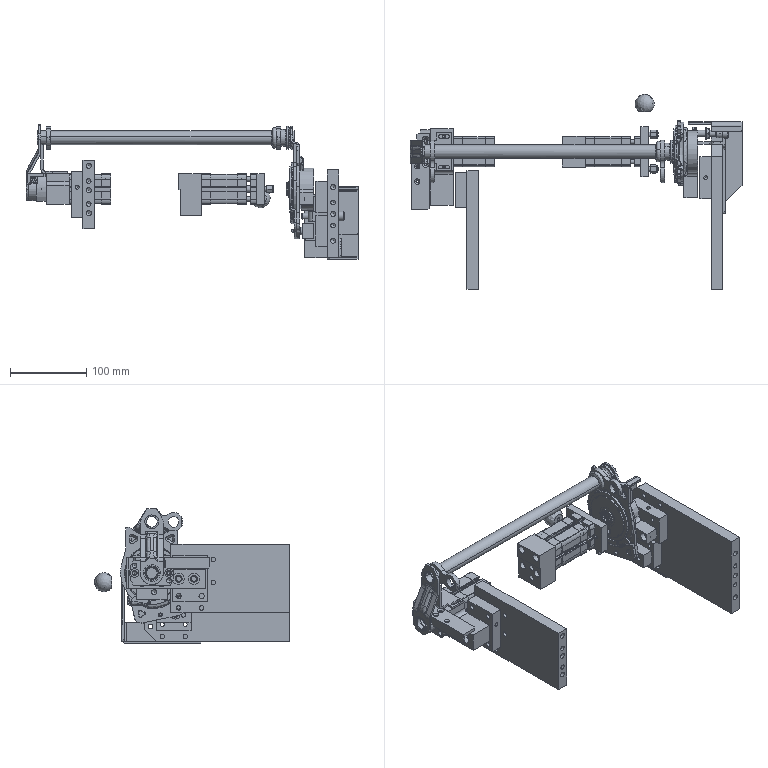Part | NX | features BREP 52 | 57 solids | 3978 faces | volume 1208582 mm3 | plane 1532 | cylinder 1439 | spline 436 | cone 309 | torus 227 | sphere 35 | commonest cylinder face diameters 0.3 x169 0.6 x144 6 x73 1 x66 0.8 x62 1.6 x58